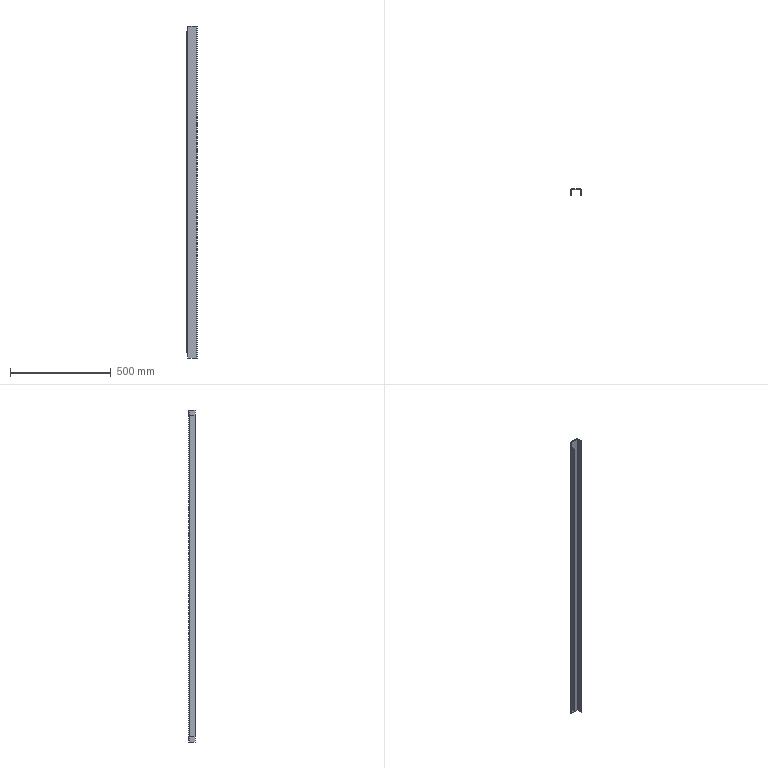Part | SolidWorks | 1 solid | 26 faces | box 50 x 30 x 1644 mm | volume 501398 mm3 | plane 22 | cylinder 4 | commonest cylinder face diameters 0.2 x2 6.2 x2
STEP:
#1=CARTESIAN_POINT('',(-25.,-3.1,795.));
#2=VERTEX_POINT('',#1);
#3=CARTESIAN_POINT('',(-25.,-30.,795.));
#4=VERTEX_POINT('',#3);
#5=CARTESIAN_POINT('',(-25.,-30.,795.));
#6=DIRECTION('',(0.,-1.,0.));
#7=VECTOR('',#6,1000.);
#8=LINE('',#5,#7);
#9=EDGE_CURVE('',#2,#4,#8,.T.);
#10=ORIENTED_EDGE('',*,*,#9,.F.);
#11=CARTESIAN_POINT('',(-25.,-3.1,-795.));
#12=VERTEX_POINT('',#11);
#13=CARTESIAN_POINT('',(-25.,-3.1,-822.));
#14=DIRECTION('',(0.,0.,1.));
#15=VECTOR('',#14,1000.);
#16=LINE('',#13,#15);
#17=EDGE_CURVE('',#12,#2,#16,.T.);
#18=ORIENTED_EDGE('',*,*,#17,.F.);
#19=CARTESIAN_POINT('',(-25.,-30.,-795.));
#20=VERTEX_POINT('',#19);
#21=CARTESIAN_POINT('',(-25.,-30.,-795.));
#22=DIRECTION('',(0.,-1.,0.));
#23=VECTOR('',#22,1000.);
#24=LINE('',#21,#23);
#25=EDGE_CURVE('',#12,#20,#24,.T.);
#26=ORIENTED_EDGE('',*,*,#25,.T.);
#27=CARTESIAN_POINT('',(-25.,-30.,-822.));
#28=DIRECTION('',(0.,0.,1.));
#29=VECTOR('',#28,1000.);
#30=LINE('',#27,#29);
#31=EDGE_CURVE('',#20,#4,#30,.T.);
#32=ORIENTED_EDGE('',*,*,#31,.T.);
#33=EDGE_LOOP('',(#10,#18,#26,#32));
#34=FACE_OUTER_BOUND('',#33,.T.);
#35=CARTESIAN_POINT('',(-25.,0.,-822.));
#36=DIRECTION('',(1.,0.,0.));
#37=DIRECTION('',(0.,0.,1.));
#38=AXIS2_PLACEMENT_3D('',#35,#36,#37);
#39=PLANE('',#38);
#40=ADVANCED_FACE('',(#34),#39,.F.);
#41=ORIENTED_EDGE('',*,*,#31,.F.);
#42=CARTESIAN_POINT('',(-22.,-30.,-795.));
#43=VERTEX_POINT('',#42);
#44=CARTESIAN_POINT('',(-25.,-30.,-795.));
#45=DIRECTION('',(1.,0.,0.));
#46=VECTOR('',#45,1000.);
#47=LINE('',#44,#46);
#48=EDGE_CURVE('',#20,#43,#47,.T.);
#49=ORIENTED_EDGE('',*,*,#48,.T.);
#50=CARTESIAN_POINT('',(-22.,-30.,795.));
#51=VERTEX_POINT('',#50);
#52=CARTESIAN_POINT('',(-22.,-30.,-822.));
#53=DIRECTION('',(0.,0.,1.));
#54=VECTOR('',#53,1000.);
#55=LINE('',#52,#54);
#56=EDGE_CURVE('',#43,#51,#55,.T.);
#57=ORIENTED_EDGE('',*,*,#56,.T.);
#58=CARTESIAN_POINT('',(-25.,-30.,795.));
#59=DIRECTION('',(1.,0.,0.));
#60=VECTOR('',#59,1000.);
#61=LINE('',#58,#60);
#62=EDGE_CURVE('',#4,#51,#61,.T.);
#63=ORIENTED_EDGE('',*,*,#62,.F.);
#64=EDGE_LOOP('',(#41,#49,#57,#63));
#65=FACE_OUTER_BOUND('',#64,.T.);
#66=CARTESIAN_POINT('',(-22.,-30.,-822.));
#67=DIRECTION('',(0.,-1.,0.));
#68=DIRECTION('',(0.,0.,1.));
#69=AXIS2_PLACEMENT_3D('',#66,#67,#68);
#70=PLANE('',#69);
#71=ADVANCED_FACE('',(#65),#70,.T.);
#72=ORIENTED_EDGE('',*,*,#56,.F.);
#73=CARTESIAN_POINT('',(-22.,-3.1,-795.));
#74=VERTEX_POINT('',#73);
#75=CARTESIAN_POINT('',(-22.,0.,-795.));
#76=DIRECTION('',(0.,-1.,0.));
#77=VECTOR('',#76,1000.);
#78=LINE('',#75,#77);
#79=EDGE_CURVE('',#74,#43,#78,.T.);
#80=ORIENTED_EDGE('',*,*,#79,.F.);
#81=CARTESIAN_POINT('',(-22.,-3.1,795.));
#82=VERTEX_POINT('',#81);
#83=CARTESIAN_POINT('',(-22.,-3.1,-822.));
#84=DIRECTION('',(0.,0.,1.));
#85=VECTOR('',#84,1000.);
#86=LINE('',#83,#85);
#87=EDGE_CURVE('',#74,#82,#86,.T.);
#88=ORIENTED_EDGE('',*,*,#87,.T.);
#89=CARTESIAN_POINT('',(-22.,0.,795.));
#90=DIRECTION('',(0.,-1.,0.));
#91=VECTOR('',#90,1000.);
#92=LINE('',#89,#91);
#93=EDGE_CURVE('',#82,#51,#92,.T.);
#94=ORIENTED_EDGE('',*,*,#93,.T.);
#95=EDGE_LOOP('',(#72,#80,#88,#94));
#96=FACE_OUTER_BOUND('',#95,.T.);
#97=CARTESIAN_POINT('',(-22.,0.,-822.));
#98=DIRECTION('',(1.,0.,0.));
#99=DIRECTION('',(0.,0.,1.));
#100=AXIS2_PLACEMENT_3D('',#97,#98,#99);
#101=PLANE('',#100);
#102=ADVANCED_FACE('',(#96),#101,.T.);
#103=CARTESIAN_POINT('',(-21.903,-3.,795.));
#104=VERTEX_POINT('',#103);
#105=CARTESIAN_POINT('',(-21.9,-3.1,795.));
#106=DIRECTION('',(0.,0.,-1.));
#107=DIRECTION('',(-1.,0.,0.));
#108=AXIS2_PLACEMENT_3D('',#105,#106,#107);
#109=CIRCLE('',#108,0.1);
#110=EDGE_CURVE('',#82,#104,#109,.T.);
#111=ORIENTED_EDGE('',*,*,#110,.F.);
#112=ORIENTED_EDGE('',*,*,#87,.F.);
#113=CARTESIAN_POINT('',(-21.903,-3.,-795.));
#114=VERTEX_POINT('',#113);
#115=CARTESIAN_POINT('',(-21.9,-3.1,-795.));
#116=DIRECTION('',(0.,0.,-1.));
#117=DIRECTION('',(-1.,0.,0.));
#118=AXIS2_PLACEMENT_3D('',#115,#116,#117);
#119=CIRCLE('',#118,0.1);
#120=EDGE_CURVE('',#74,#114,#119,.T.);
#121=ORIENTED_EDGE('',*,*,#120,.T.);
#122=CARTESIAN_POINT('',(-21.903,-3.,-822.));
#123=VERTEX_POINT('',#122);
#124=CARTESIAN_POINT('',(-21.903,-3.,-822.));
#125=DIRECTION('',(0.,0.,1.));
#126=VECTOR('',#125,1000.);
#127=LINE('',#124,#126);
#128=EDGE_CURVE('',#123,#114,#127,.T.);
#129=ORIENTED_EDGE('',*,*,#128,.F.);
#130=CARTESIAN_POINT('',(-21.9,-3.,-822.));
#131=VERTEX_POINT('',#130);
#132=CARTESIAN_POINT('',(-21.9,-3.1,-822.));
#133=DIRECTION('',(0.,0.,1.));
#134=DIRECTION('',(1.,0.,0.));
#135=AXIS2_PLACEMENT_3D('',#132,#133,#134);
#136=CIRCLE('',#135,0.1);
#137=EDGE_CURVE('',#131,#123,#136,.T.);
#138=ORIENTED_EDGE('',*,*,#137,.F.);
#139=CARTESIAN_POINT('',(-21.9,-3.,822.));
#140=VERTEX_POINT('',#139);
#141=CARTESIAN_POINT('',(-21.9,-3.,-822.));
#142=DIRECTION('',(0.,0.,1.));
#143=VECTOR('',#142,1000.);
#144=LINE('',#141,#143);
#145=EDGE_CURVE('',#131,#140,#144,.T.);
#146=ORIENTED_EDGE('',*,*,#145,.T.);
#147=CARTESIAN_POINT('',(-21.903,-3.,822.));
#148=VERTEX_POINT('',#147);
#149=CARTESIAN_POINT('',(-21.9,-3.1,822.));
#150=DIRECTION('',(0.,0.,1.));
#151=DIRECTION('',(1.,0.,0.));
#152=AXIS2_PLACEMENT_3D('',#149,#150,#151);
#153=CIRCLE('',#152,0.1);
#154=EDGE_CURVE('',#140,#148,#153,.T.);
#155=ORIENTED_EDGE('',*,*,#154,.T.);
#156=CARTESIAN_POINT('',(-21.903,-3.,-822.));
#157=DIRECTION('',(0.,0.,1.));
#158=VECTOR('',#157,1000.);
#159=LINE('',#156,#158);
#160=EDGE_CURVE('',#104,#148,#159,.T.);
#161=ORIENTED_EDGE('',*,*,#160,.F.);
#162=EDGE_LOOP('',(#111,#112,#121,#129,#138,#146,#155,#161));
#163=FACE_OUTER_BOUND('',#162,.T.);
#164=CARTESIAN_POINT('',(-21.9,-3.1,-822.));
#165=DIRECTION('',(0.,0.,1.));
#166=DIRECTION('',(-1.,0.,0.));
#167=AXIS2_PLACEMENT_3D('',#164,#165,#166);
#168=CYLINDRICAL_SURFACE('',#167,0.1);
#169=ADVANCED_FACE('',(#163),#168,.F.);
#170=CARTESIAN_POINT('',(-22.,-0.001613,795.));
#171=VERTEX_POINT('',#170);
#172=CARTESIAN_POINT('',(-22.,-0.001613,822.));
#173=VERTEX_POINT('',#172);
#174=CARTESIAN_POINT('',(-22.,-0.001613,-822.));
#175=DIRECTION('',(0.,0.,1.));
#176=VECTOR('',#175,1000.);
#177=LINE('',#174,#176);
#178=EDGE_CURVE('',#171,#173,#177,.T.);
#179=ORIENTED_EDGE('',*,*,#178,.T.);
#180=CARTESIAN_POINT('',(-21.9,0.,822.));
#181=VERTEX_POINT('',#180);
#182=CARTESIAN_POINT('',(-21.9,-3.1,822.));
#183=DIRECTION('',(0.,0.,1.));
#184=DIRECTION('',(-1.,0.,0.));
#185=AXIS2_PLACEMENT_3D('',#182,#183,#184);
#186=CIRCLE('',#185,3.1);
#187=EDGE_CURVE('',#181,#173,#186,.T.);
#188=ORIENTED_EDGE('',*,*,#187,.F.);
#189=CARTESIAN_POINT('',(-21.9,0.,-822.));
#190=VERTEX_POINT('',#189);
#191=CARTESIAN_POINT('',(-21.9,0.,-822.));
#192=DIRECTION('',(0.,0.,1.));
#193=VECTOR('',#192,1000.);
#194=LINE('',#191,#193);
#195=EDGE_CURVE('',#190,#181,#194,.T.);
#196=ORIENTED_EDGE('',*,*,#195,.F.);
#197=CARTESIAN_POINT('',(-22.,-0.001613,-822.));
#198=VERTEX_POINT('',#197);
#199=CARTESIAN_POINT('',(-21.9,-3.1,-822.));
#200=DIRECTION('',(0.,0.,1.));
#201=DIRECTION('',(-1.,0.,0.));
#202=AXIS2_PLACEMENT_3D('',#199,#200,#201);
#203=CIRCLE('',#202,3.1);
#204=EDGE_CURVE('',#190,#198,#203,.T.);
#205=ORIENTED_EDGE('',*,*,#204,.T.);
#206=CARTESIAN_POINT('',(-22.,-0.001613,-795.));
#207=VERTEX_POINT('',#206);
#208=CARTESIAN_POINT('',(-22.,-0.001613,-822.));
#209=DIRECTION('',(0.,0.,1.));
#210=VECTOR('',#209,1000.);
#211=LINE('',#208,#210);
#212=EDGE_CURVE('',#198,#207,#211,.T.);
#213=ORIENTED_EDGE('',*,*,#212,.T.);
#214=CARTESIAN_POINT('',(-21.9,-3.1,-795.));
#215=DIRECTION('',(0.,0.,-1.));
#216=DIRECTION('',(-1.,0.,0.));
#217=AXIS2_PLACEMENT_3D('',#214,#215,#216);
#218=CIRCLE('',#217,3.1);
#219=EDGE_CURVE('',#12,#207,#218,.T.);
#220=ORIENTED_EDGE('',*,*,#219,.F.);
#221=ORIENTED_EDGE('',*,*,#17,.T.);
#222=CARTESIAN_POINT('',(-21.9,-3.1,795.));
#223=DIRECTION('',(0.,0.,-1.));
#224=DIRECTION('',(-1.,0.,0.));
#225=AXIS2_PLACEMENT_3D('',#222,#223,#224);
#226=CIRCLE('',#225,3.1);
#227=EDGE_CURVE('',#2,#171,#226,.T.);
#228=ORIENTED_EDGE('',*,*,#227,.T.);
#229=EDGE_LOOP('',(#179,#188,#196,#205,#213,#220,#221,#228));
#230=FACE_OUTER_BOUND('',#229,.T.);
#231=CARTESIAN_POINT('',(-21.9,-3.1,-822.));
#232=DIRECTION('',(0.,0.,1.));
#233=DIRECTION('',(-1.,0.,0.));
#234=AXIS2_PLACEMENT_3D('',#231,#232,#233);
#235=CYLINDRICAL_SURFACE('',#234,3.1);
#236=ADVANCED_FACE('',(#230),#235,.T.);
#237=ORIENTED_EDGE('',*,*,#154,.F.);
#238=CARTESIAN_POINT('',(-21.9,-3.,822.));
#239=DIRECTION('',(0.,1.,0.));
#240=VECTOR('',#239,1000.);
#241=LINE('',#238,#240);
#242=EDGE_CURVE('',#140,#181,#241,.T.);
#243=ORIENTED_EDGE('',*,*,#242,.T.);
#244=ORIENTED_EDGE('',*,*,#187,.T.);
#245=CARTESIAN_POINT('',(-22.,-0.001613,822.));
#246=DIRECTION('',(0.03226,-0.9995,0.));
#247=VECTOR('',#246,1000.);
#248=LINE('',#245,#247);
#249=EDGE_CURVE('',#173,#148,#248,.T.);
#250=ORIENTED_EDGE('',*,*,#249,.T.);
#251=EDGE_LOOP('',(#237,#243,#244,#250));
#252=FACE_OUTER_BOUND('',#251,.T.);
#253=CARTESIAN_POINT('',(-25.,-3.1,822.));
#254=DIRECTION('',(0.,0.,1.));
#255=DIRECTION('',(-1.,0.,0.));
#256=AXIS2_PLACEMENT_3D('',#253,#254,#255);
#257=PLANE('',#256);
#258=ADVANCED_FACE('',(#252),#257,.T.);
#259=ORIENTED_EDGE('',*,*,#204,.F.);
#260=CARTESIAN_POINT('',(-21.9,0.,-822.));
#261=DIRECTION('',(0.,-1.,0.));
#262=VECTOR('',#261,1000.);
#263=LINE('',#260,#262);
#264=EDGE_CURVE('',#190,#131,#263,.T.);
#265=ORIENTED_EDGE('',*,*,#264,.T.);
#266=ORIENTED_EDGE('',*,*,#137,.T.);
#267=CARTESIAN_POINT('',(-22.,-0.001613,-822.));
#268=DIRECTION('',(0.03226,-0.9995,0.));
#269=VECTOR('',#268,1000.);
#270=LINE('',#267,#269);
#271=EDGE_CURVE('',#198,#123,#270,.T.);
#272=ORIENTED_EDGE('',*,*,#271,.F.);
#273=EDGE_LOOP('',(#259,#265,#266,#272));
#274=FACE_OUTER_BOUND('',#273,.T.);
#275=CARTESIAN_POINT('',(-21.9,0.,-822.));
#276=DIRECTION('',(0.,0.,-1.));
#277=DIRECTION('',(1.,0.,0.));
#278=AXIS2_PLACEMENT_3D('',#275,#276,#277);
#279=PLANE('',#278);
#280=ADVANCED_FACE('',(#274),#279,.T.);
#281=CARTESIAN_POINT('',(25.,-3.1,-822.));
#282=VERTEX_POINT('',#281);
#283=CARTESIAN_POINT('',(22.,-3.1,-822.));
#284=VERTEX_POINT('',#283);
#285=CARTESIAN_POINT('',(25.,-3.1,-822.));
#286=DIRECTION('',(-1.,0.,0.));
#287=VECTOR('',#286,1000.);
#288=LINE('',#285,#287);
#289=EDGE_CURVE('',#282,#284,#288,.T.);
#290=ORIENTED_EDGE('',*,*,#289,.T.);
#291=CARTESIAN_POINT('',(21.9,-3.,-822.));
#292=VERTEX_POINT('',#291);
#293=CARTESIAN_POINT('',(21.9,-3.1,-822.));
#294=DIRECTION('',(0.,0.,1.));
#295=DIRECTION('',(1.,0.,0.));
#296=AXIS2_PLACEMENT_3D('',#293,#294,#295);
#297=CIRCLE('',#296,0.1);
#298=EDGE_CURVE('',#284,#292,#297,.T.);
#299=ORIENTED_EDGE('',*,*,#298,.T.);
#300=CARTESIAN_POINT('',(21.9,0.,-822.));
#301=VERTEX_POINT('',#300);
#302=CARTESIAN_POINT('',(21.9,-3.,-822.));
#303=DIRECTION('',(0.,1.,0.));
#304=VECTOR('',#303,1000.);
#305=LINE('',#302,#304);
#306=EDGE_CURVE('',#292,#301,#305,.T.);
#307=ORIENTED_EDGE('',*,*,#306,.T.);
#308=CARTESIAN_POINT('',(21.9,-3.1,-822.));
#309=DIRECTION('',(0.,0.,1.));
#310=DIRECTION('',(-1.,0.,0.));
#311=AXIS2_PLACEMENT_3D('',#308,#309,#310);
#312=CIRCLE('',#311,3.1);
#313=EDGE_CURVE('',#282,#301,#312,.T.);
#314=ORIENTED_EDGE('',*,*,#313,.F.);
#315=EDGE_LOOP('',(#290,#299,#307,#314));
#316=FACE_OUTER_BOUND('',#315,.T.);
#317=CARTESIAN_POINT('',(25.,-3.1,-822.));
#318=DIRECTION('',(0.,0.,-1.));
#319=DIRECTION('',(1.,0.,0.));
#320=AXIS2_PLACEMENT_3D('',#317,#318,#319);
#321=PLANE('',#320);
#322=ADVANCED_FACE('',(#316),#321,.T.);
#323=CARTESIAN_POINT('',(25.,-30.,-822.));
#324=VERTEX_POINT('',#323);
#325=CARTESIAN_POINT('',(25.,0.,-822.));
#326=DIRECTION('',(0.,1.,0.));
#327=VECTOR('',#326,1000.);
#328=LINE('',#325,#327);
#329=EDGE_CURVE('',#324,#282,#328,.T.);
#330=ORIENTED_EDGE('',*,*,#329,.F.);
#331=CARTESIAN_POINT('',(22.,-30.,-822.));
#332=VERTEX_POINT('',#331);
#333=CARTESIAN_POINT('',(25.,-30.,-822.));
#334=DIRECTION('',(-1.,0.,0.));
#335=VECTOR('',#334,1000.);
#336=LINE('',#333,#335);
#337=EDGE_CURVE('',#324,#332,#336,.T.);
#338=ORIENTED_EDGE('',*,*,#337,.T.);
#339=CARTESIAN_POINT('',(22.,0.,-822.));
#340=DIRECTION('',(0.,1.,0.));
#341=VECTOR('',#340,1000.);
#342=LINE('',#339,#341);
#343=EDGE_CURVE('',#332,#284,#342,.T.);
#344=ORIENTED_EDGE('',*,*,#343,.T.);
#345=ORIENTED_EDGE('',*,*,#289,.F.);
#346=EDGE_LOOP('',(#330,#338,#344,#345));
#347=FACE_OUTER_BOUND('',#346,.T.);
#348=CARTESIAN_POINT('',(21.9,-3.,-822.));
#349=DIRECTION('',(0.,0.,-1.));
#350=DIRECTION('',(1.,0.,0.));
#351=AXIS2_PLACEMENT_3D('',#348,#349,#350);
#352=PLANE('',#351);
#353=ADVANCED_FACE('',(#347),#352,.T.);
#354=CARTESIAN_POINT('',(21.9,0.,822.));
#355=VERTEX_POINT('',#354);
#356=CARTESIAN_POINT('',(21.9,-3.,822.));
#357=VERTEX_POINT('',#356);
#358=CARTESIAN_POINT('',(21.9,0.,822.));
#359=DIRECTION('',(0.,-1.,0.));
#360=VECTOR('',#359,1000.);
#361=LINE('',#358,#360);
#362=EDGE_CURVE('',#355,#357,#361,.T.);
#363=ORIENTED_EDGE('',*,*,#362,.T.);
#364=CARTESIAN_POINT('',(22.,-3.1,822.));
#365=VERTEX_POINT('',#364);
#366=CARTESIAN_POINT('',(21.9,-3.1,822.));
#367=DIRECTION('',(0.,0.,1.));
#368=DIRECTION('',(1.,0.,0.));
#369=AXIS2_PLACEMENT_3D('',#366,#367,#368);
#370=CIRCLE('',#369,0.1);
#371=EDGE_CURVE('',#365,#357,#370,.T.);
#372=ORIENTED_EDGE('',*,*,#371,.F.);
#373=CARTESIAN_POINT('',(25.,-3.1,822.));
#374=VERTEX_POINT('',#373);
#375=CARTESIAN_POINT('',(22.,-3.1,822.));
#376=DIRECTION('',(1.,0.,0.));
#377=VECTOR('',#376,1000.);
#378=LINE('',#375,#377);
#379=EDGE_CURVE('',#365,#374,#378,.T.);
#380=ORIENTED_EDGE('',*,*,#379,.T.);
#381=CARTESIAN_POINT('',(21.9,-3.1,822.));
#382=DIRECTION('',(0.,0.,1.));
#383=DIRECTION('',(-1.,0.,0.));
#384=AXIS2_PLACEMENT_3D('',#381,#382,#383);
#385=CIRCLE('',#384,3.1);
#386=EDGE_CURVE('',#374,#355,#385,.T.);
#387=ORIENTED_EDGE('',*,*,#386,.T.);
#388=EDGE_LOOP('',(#363,#372,#380,#387));
#389=FACE_OUTER_BOUND('',#388,.T.);
#390=CARTESIAN_POINT('',(21.9,0.,822.));
#391=DIRECTION('',(0.,0.,1.));
#392=DIRECTION('',(-1.,0.,0.));
#393=AXIS2_PLACEMENT_3D('',#390,#391,#392);
#394=PLANE('',#393);
#395=ADVANCED_FACE('',(#389),#394,.T.);
#396=CARTESIAN_POINT('',(-25.,0.,822.));
#397=DIRECTION('',(-1.,0.,0.));
#398=VECTOR('',#397,1000.);
#399=LINE('',#396,#398);
#400=EDGE_CURVE('',#355,#181,#399,.T.);
#401=ORIENTED_EDGE('',*,*,#400,.T.);
#402=ORIENTED_EDGE('',*,*,#242,.F.);
#403=CARTESIAN_POINT('',(-25.,-3.,822.));
#404=DIRECTION('',(-1.,0.,0.));
#405=VECTOR('',#404,1000.);
#406=LINE('',#403,#405);
#407=EDGE_CURVE('',#357,#140,#406,.T.);
#408=ORIENTED_EDGE('',*,*,#407,.F.);
#409=ORIENTED_EDGE('',*,*,#362,.F.);
#410=EDGE_LOOP('',(#401,#402,#408,#409));
#411=FACE_OUTER_BOUND('',#410,.T.);
#412=CARTESIAN_POINT('',(22.,-3.1,822.));
#413=DIRECTION('',(0.,0.,1.));
#414=DIRECTION('',(-1.,0.,0.));
#415=AXIS2_PLACEMENT_3D('',#412,#413,#414);
#416=PLANE('',#415);
#417=ADVANCED_FACE('',(#411),#416,.T.);
#418=CARTESIAN_POINT('',(-25.,0.,-822.));
#419=DIRECTION('',(-1.,0.,0.));
#420=VECTOR('',#419,1000.);
#421=LINE('',#418,#420);
#422=EDGE_CURVE('',#301,#190,#421,.T.);
#423=ORIENTED_EDGE('',*,*,#422,.F.);
#424=ORIENTED_EDGE('',*,*,#306,.F.);
#425=CARTESIAN_POINT('',(-25.,-3.,-822.));
#426=DIRECTION('',(-1.,0.,0.));
#427=VECTOR('',#426,1000.);
#428=LINE('',#425,#427);
#429=EDGE_CURVE('',#292,#131,#428,.T.);
#430=ORIENTED_EDGE('',*,*,#429,.T.);
#431=ORIENTED_EDGE('',*,*,#264,.F.);
#432=EDGE_LOOP('',(#423,#424,#430,#431));
#433=FACE_OUTER_BOUND('',#432,.T.);
#434=CARTESIAN_POINT('',(-22.,-3.1,-822.));
#435=DIRECTION('',(0.,0.,-1.));
#436=DIRECTION('',(1.,0.,0.));
#437=AXIS2_PLACEMENT_3D('',#434,#435,#436);
#438=PLANE('',#437);
#439=ADVANCED_FACE('',(#433),#438,.T.);
#440=ORIENTED_EDGE('',*,*,#407,.T.);
#441=ORIENTED_EDGE('',*,*,#145,.F.);
#442=ORIENTED_EDGE('',*,*,#429,.F.);
#443=CARTESIAN_POINT('',(21.9,-3.,-822.));
#444=DIRECTION('',(0.,0.,1.));
#445=VECTOR('',#444,1000.);
#446=LINE('',#443,#445);
#447=EDGE_CURVE('',#292,#357,#446,.T.);
#448=ORIENTED_EDGE('',*,*,#447,.T.);
#449=EDGE_LOOP('',(#440,#441,#442,#448));
#450=FACE_OUTER_BOUND('',#449,.T.);
#451=CARTESIAN_POINT('',(-25.,-3.,-822.));
#452=DIRECTION('',(0.,-1.,0.));
#453=DIRECTION('',(1.,0.,0.));
#454=AXIS2_PLACEMENT_3D('',#451,#452,#453);
#455=PLANE('',#454);
#456=ADVANCED_FACE('',(#450),#455,.T.);
#457=ORIENTED_EDGE('',*,*,#371,.T.);
#458=ORIENTED_EDGE('',*,*,#447,.F.);
#459=ORIENTED_EDGE('',*,*,#298,.F.);
#460=CARTESIAN_POINT('',(22.,-3.1,-822.));
#461=DIRECTION('',(0.,0.,1.));
#462=VECTOR('',#461,1000.);
#463=LINE('',#460,#462);
#464=EDGE_CURVE('',#284,#365,#463,.T.);
#465=ORIENTED_EDGE('',*,*,#464,.T.);
#466=EDGE_LOOP('',(#457,#458,#459,#465));
#467=FACE_OUTER_BOUND('',#466,.T.);
#468=CARTESIAN_POINT('',(21.9,-3.1,-822.));
#469=DIRECTION('',(0.,0.,1.));
#470=DIRECTION('',(-1.,0.,0.));
#471=AXIS2_PLACEMENT_3D('',#468,#469,#470);
#472=CYLINDRICAL_SURFACE('',#471,0.1);
#473=ADVANCED_FACE('',(#467),#472,.F.);
#474=CARTESIAN_POINT('',(22.,-30.,822.));
#475=VERTEX_POINT('',#474);
#476=CARTESIAN_POINT('',(22.,0.,822.));
#477=DIRECTION('',(0.,1.,0.));
#478=VECTOR('',#477,1000.);
#479=LINE('',#476,#478);
#480=EDGE_CURVE('',#475,#365,#479,.T.);
#481=ORIENTED_EDGE('',*,*,#480,.T.);
#482=ORIENTED_EDGE('',*,*,#464,.F.);
#483=ORIENTED_EDGE('',*,*,#343,.F.);
#484=CARTESIAN_POINT('',(22.,-30.,-822.));
#485=DIRECTION('',(0.,0.,1.));
#486=VECTOR('',#485,1000.);
#487=LINE('',#484,#486);
#488=EDGE_CURVE('',#332,#475,#487,.T.);
#489=ORIENTED_EDGE('',*,*,#488,.T.);
#490=EDGE_LOOP('',(#481,#482,#483,#489));
#491=FACE_OUTER_BOUND('',#490,.T.);
#492=CARTESIAN_POINT('',(22.,0.,-822.));
#493=DIRECTION('',(-1.,0.,0.));
#494=DIRECTION('',(0.,-1.,0.));
#495=AXIS2_PLACEMENT_3D('',#492,#493,#494);
#496=PLANE('',#495);
#497=ADVANCED_FACE('',(#491),#496,.T.);
#498=CARTESIAN_POINT('',(25.,-30.,822.));
#499=VERTEX_POINT('',#498);
#500=CARTESIAN_POINT('',(25.,-30.,822.));
#501=DIRECTION('',(-1.,0.,0.));
#502=VECTOR('',#501,1000.);
#503=LINE('',#500,#502);
#504=EDGE_CURVE('',#499,#475,#503,.T.);
#505=ORIENTED_EDGE('',*,*,#504,.T.);
#506=ORIENTED_EDGE('',*,*,#488,.F.);
#507=ORIENTED_EDGE('',*,*,#337,.F.);
#508=CARTESIAN_POINT('',(25.,-30.,-822.));
#509=DIRECTION('',(0.,0.,1.));
#510=VECTOR('',#509,1000.);
#511=LINE('',#508,#510);
#512=EDGE_CURVE('',#324,#499,#511,.T.);
#513=ORIENTED_EDGE('',*,*,#512,.T.);
#514=EDGE_LOOP('',(#505,#506,#507,#513));
#515=FACE_OUTER_BOUND('',#514,.T.);
#516=CARTESIAN_POINT('',(25.,-30.,-822.));
#517=DIRECTION('',(0.,-1.,0.));
#518=DIRECTION('',(1.,0.,0.));
#519=AXIS2_PLACEMENT_3D('',#516,#517,#518);
#520=PLANE('',#519);
#521=ADVANCED_FACE('',(#515),#520,.T.);
#522=CARTESIAN_POINT('',(25.,0.,822.));
#523=DIRECTION('',(0.,1.,0.));
#524=VECTOR('',#523,1000.);
#525=LINE('',#522,#524);
#526=EDGE_CURVE('',#499,#374,#525,.T.);
#527=ORIENTED_EDGE('',*,*,#526,.F.);
#528=ORIENTED_EDGE('',*,*,#512,.F.);
#529=ORIENTED_EDGE('',*,*,#329,.T.);
#530=CARTESIAN_POINT('',(25.,-3.1,-822.));
#531=DIRECTION('',(0.,0.,1.));
#532=VECTOR('',#531,1000.);
#533=LINE('',#530,#532);
#534=EDGE_CURVE('',#282,#374,#533,.T.);
#535=ORIENTED_EDGE('',*,*,#534,.T.);
#536=EDGE_LOOP('',(#527,#528,#529,#535));
#537=FACE_OUTER_BOUND('',#536,.T.);
#538=CARTESIAN_POINT('',(25.,0.,-822.));
#539=DIRECTION('',(-1.,0.,0.));
#540=DIRECTION('',(0.,-1.,0.));
#541=AXIS2_PLACEMENT_3D('',#538,#539,#540);
#542=PLANE('',#541);
#543=ADVANCED_FACE('',(#537),#542,.F.);
#544=ORIENTED_EDGE('',*,*,#386,.F.);
#545=ORIENTED_EDGE('',*,*,#534,.F.);
#546=ORIENTED_EDGE('',*,*,#313,.T.);
#547=CARTESIAN_POINT('',(21.9,0.,-822.));
#548=DIRECTION('',(0.,0.,1.));
#549=VECTOR('',#548,1000.);
#550=LINE('',#547,#549);
#551=EDGE_CURVE('',#301,#355,#550,.T.);
#552=ORIENTED_EDGE('',*,*,#551,.T.);
#553=EDGE_LOOP('',(#544,#545,#546,#552));
#554=FACE_OUTER_BOUND('',#553,.T.);
#555=CARTESIAN_POINT('',(21.9,-3.1,-822.));
#556=DIRECTION('',(0.,0.,1.));
#557=DIRECTION('',(-1.,0.,0.));
#558=AXIS2_PLACEMENT_3D('',#555,#556,#557);
#559=CYLINDRICAL_SURFACE('',#558,3.1);
#560=ADVANCED_FACE('',(#554),#559,.T.);
#561=ORIENTED_EDGE('',*,*,#400,.F.);
#562=ORIENTED_EDGE('',*,*,#551,.F.);
#563=ORIENTED_EDGE('',*,*,#422,.T.);
#564=ORIENTED_EDGE('',*,*,#195,.T.);
#565=EDGE_LOOP('',(#561,#562,#563,#564));
#566=FACE_OUTER_BOUND('',#565,.T.);
#567=CARTESIAN_POINT('',(-25.,0.,-822.));
#568=DIRECTION('',(0.,-1.,0.));
#569=DIRECTION('',(1.,0.,0.));
#570=AXIS2_PLACEMENT_3D('',#567,#568,#569);
#571=PLANE('',#570);
#572=ADVANCED_FACE('',(#566),#571,.F.);
#573=ORIENTED_EDGE('',*,*,#480,.F.);
#574=ORIENTED_EDGE('',*,*,#504,.F.);
#575=ORIENTED_EDGE('',*,*,#526,.T.);
#576=ORIENTED_EDGE('',*,*,#379,.F.);
#577=EDGE_LOOP('',(#573,#574,#575,#576));
#578=FACE_OUTER_BOUND('',#577,.T.);
#579=CARTESIAN_POINT('',(-21.9,-3.1,822.));
#580=DIRECTION('',(0.,0.,-1.));
#581=DIRECTION('',(1.,0.,0.));
#582=AXIS2_PLACEMENT_3D('',#579,#580,#581);
#583=PLANE('',#582);
#584=ADVANCED_FACE('',(#578),#583,.F.);
#585=CARTESIAN_POINT('',(-25.,-3.1,-795.));
#586=DIRECTION('',(1.,0.,0.));
#587=VECTOR('',#586,1000.);
#588=LINE('',#585,#587);
#589=EDGE_CURVE('',#12,#74,#588,.T.);
#590=ORIENTED_EDGE('',*,*,#589,.T.);
#591=ORIENTED_EDGE('',*,*,#79,.T.);
#592=ORIENTED_EDGE('',*,*,#48,.F.);
#593=ORIENTED_EDGE('',*,*,#25,.F.);
#594=EDGE_LOOP('',(#590,#591,#592,#593));
#595=FACE_OUTER_BOUND('',#594,.T.);
#596=CARTESIAN_POINT('',(-25.,-30.,-795.));
#597=DIRECTION('',(0.,0.,-1.));
#598=DIRECTION('',(0.,-1.,0.));
#599=AXIS2_PLACEMENT_3D('',#596,#597,#598);
#600=PLANE('',#599);
#601=ADVANCED_FACE('',(#595),#600,.T.);
#602=ORIENTED_EDGE('',*,*,#271,.T.);
#603=ORIENTED_EDGE('',*,*,#128,.T.);
#604=CARTESIAN_POINT('',(-22.,-0.001613,-795.));
#605=DIRECTION('',(0.03226,-0.9995,0.));
#606=VECTOR('',#605,1000.);
#607=LINE('',#604,#606);
#608=EDGE_CURVE('',#207,#114,#607,.T.);
#609=ORIENTED_EDGE('',*,*,#608,.F.);
#610=ORIENTED_EDGE('',*,*,#212,.F.);
#611=EDGE_LOOP('',(#602,#603,#609,#610));
#612=FACE_OUTER_BOUND('',#611,.T.);
#613=CARTESIAN_POINT('',(-22.,-0.001613,-808.5));
#614=DIRECTION('',(0.9995,0.03226,0.));
#615=DIRECTION('',(0.,0.,1.));
#616=AXIS2_PLACEMENT_3D('',#613,#614,#615);
#617=PLANE('',#616);
#618=ADVANCED_FACE('',(#612),#617,.F.);
#619=ORIENTED_EDGE('',*,*,#608,.T.);
#620=ORIENTED_EDGE('',*,*,#120,.F.);
#621=ORIENTED_EDGE('',*,*,#589,.F.);
#622=ORIENTED_EDGE('',*,*,#219,.T.);
#623=EDGE_LOOP('',(#619,#620,#621,#622));
#624=FACE_OUTER_BOUND('',#623,.T.);
#625=CARTESIAN_POINT('',(-21.9,-3.1,-795.));
#626=DIRECTION('',(0.,0.,-1.));
#627=DIRECTION('',(1.,0.,0.));
#628=AXIS2_PLACEMENT_3D('',#625,#626,#627);
#629=PLANE('',#628);
#630=ADVANCED_FACE('',(#624),#629,.T.);
#631=ORIENTED_EDGE('',*,*,#9,.T.);
#632=ORIENTED_EDGE('',*,*,#62,.T.);
#633=ORIENTED_EDGE('',*,*,#93,.F.);
#634=CARTESIAN_POINT('',(-25.,-3.1,795.));
#635=DIRECTION('',(1.,0.,0.));
#636=VECTOR('',#635,1000.);
#637=LINE('',#634,#636);
#638=EDGE_CURVE('',#2,#82,#637,.T.);
#639=ORIENTED_EDGE('',*,*,#638,.F.);
#640=EDGE_LOOP('',(#631,#632,#633,#639));
#641=FACE_OUTER_BOUND('',#640,.T.);
#642=CARTESIAN_POINT('',(-25.,-30.,795.));
#643=DIRECTION('',(0.,0.,-1.));
#644=DIRECTION('',(0.,-1.,0.));
#645=AXIS2_PLACEMENT_3D('',#642,#643,#644);
#646=PLANE('',#645);
#647=ADVANCED_FACE('',(#641),#646,.F.);
#648=CARTESIAN_POINT('',(-22.,-0.001613,795.));
#649=DIRECTION('',(0.03226,-0.9995,0.));
#650=VECTOR('',#649,1000.);
#651=LINE('',#648,#650);
#652=EDGE_CURVE('',#171,#104,#651,.T.);
#653=ORIENTED_EDGE('',*,*,#652,.T.);
#654=ORIENTED_EDGE('',*,*,#160,.T.);
#655=ORIENTED_EDGE('',*,*,#249,.F.);
#656=ORIENTED_EDGE('',*,*,#178,.F.);
#657=EDGE_LOOP('',(#653,#654,#655,#656));
#658=FACE_OUTER_BOUND('',#657,.T.);
#659=CARTESIAN_POINT('',(-22.,-0.001613,808.5));
#660=DIRECTION('',(0.9995,0.03226,0.));
#661=DIRECTION('',(0.,0.,1.));
#662=AXIS2_PLACEMENT_3D('',#659,#660,#661);
#663=PLANE('',#662);
#664=ADVANCED_FACE('',(#658),#663,.F.);
#665=ORIENTED_EDGE('',*,*,#227,.F.);
#666=ORIENTED_EDGE('',*,*,#638,.T.);
#667=ORIENTED_EDGE('',*,*,#110,.T.);
#668=ORIENTED_EDGE('',*,*,#652,.F.);
#669=EDGE_LOOP('',(#665,#666,#667,#668));
#670=FACE_OUTER_BOUND('',#669,.T.);
#671=CARTESIAN_POINT('',(-21.9,-3.1,795.));
#672=DIRECTION('',(0.,0.,-1.));
#673=DIRECTION('',(1.,0.,0.));
#674=AXIS2_PLACEMENT_3D('',#671,#672,#673);
#675=PLANE('',#674);
#676=ADVANCED_FACE('',(#670),#675,.F.);
#677=CLOSED_SHELL('',(#40,#71,#102,#169,#236,#258,#280,#322,#353,#395,#417,#439,#456,#473,#497,#521,#543,#560,#572,#584,#601,#618,#630,#647,#664,#676));
#678=MANIFOLD_SOLID_BREP('',#677);
#679=CARTESIAN_POINT('',(0.,0.,0.));
#680=DIRECTION('',(0.,0.,1.));
#681=DIRECTION('',(1.,0.,0.));
#682=AXIS2_PLACEMENT_3D('',#679,#680,#681);
#683=(LENGTH_UNIT()NAMED_UNIT(*)SI_UNIT(.MILLI.,.METRE.));
#684=UNCERTAINTY_MEASURE_WITH_UNIT(LENGTH_MEASURE(0.00001),#683,'','');
#685=(NAMED_UNIT(*)PLANE_ANGLE_UNIT()SI_UNIT($,.RADIAN.));
#686=(NAMED_UNIT(*)SI_UNIT($,.STERADIAN.)SOLID_ANGLE_UNIT());
#687=(GEOMETRIC_REPRESENTATION_CONTEXT(3)GLOBAL_UNCERTAINTY_ASSIGNED_CONTEXT((#684))GLOBAL_UNIT_ASSIGNED_CONTEXT((#683,#685,#686))REPRESENTATION_CONTEXT('',''));
#688=ADVANCED_BREP_SHAPE_REPRESENTATION('',(#678,#682),#687);